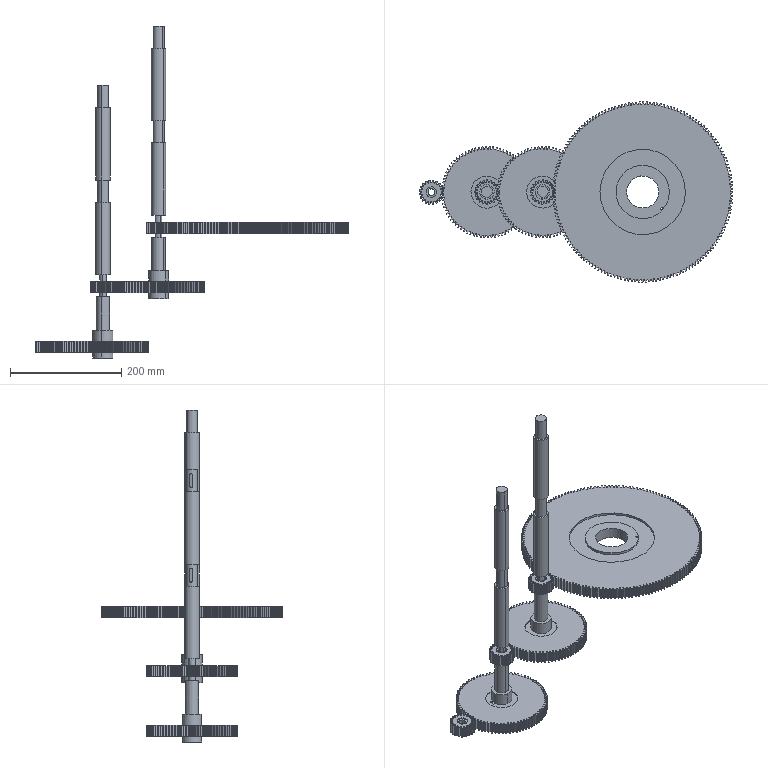Part | SolidWorks | features CompositeCurve 6, RefAxis 4, AEMSimFeature 1 | 12 solids | 2774 faces | box 563.839 x 324 x 596.9 mm | volume 2766981 mm3 | cylinder 1797 | spline 760 | plane 217 | commonest cylinder face diameters 1.52 x922 155 x162 315 x161 164 x160 324 x160 35 x63